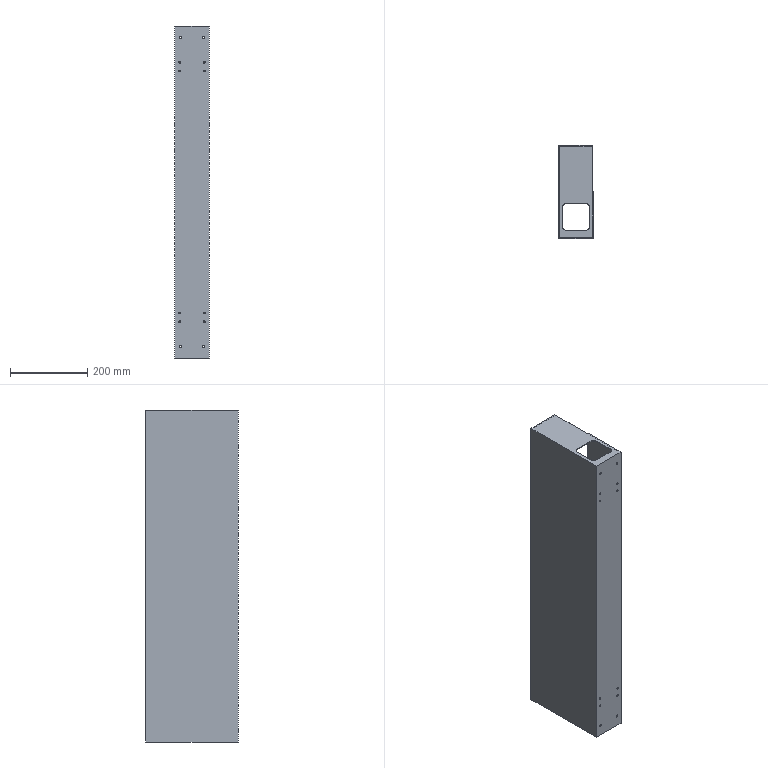Part | NX | 1 solid | 53 faces | box 90 x 240 x 860 mm | volume 844899 mm3 | cylinder 27 | plane 26 | commonest cylinder face diameters 4.2 x8 20 x8 2.5 x7 6 x4